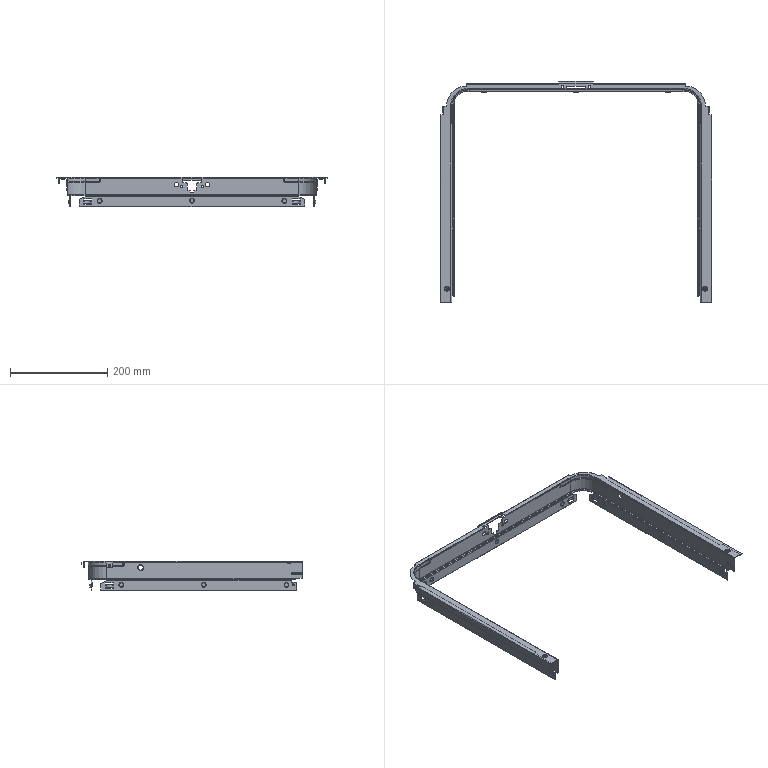Part | STEP file | ZXW722-L-03 | 1 solid | 609 faces | box 558 x 455.25 x 60 mm | volume 116020 mm3 | cylinder 258 | plane 203 | torus 68 | cone 48 | spline 24 | sphere 8 | commonest cylinder face diameters 2 x74 4 x56 10 x22 8 x18 3 x16 0.4 x8